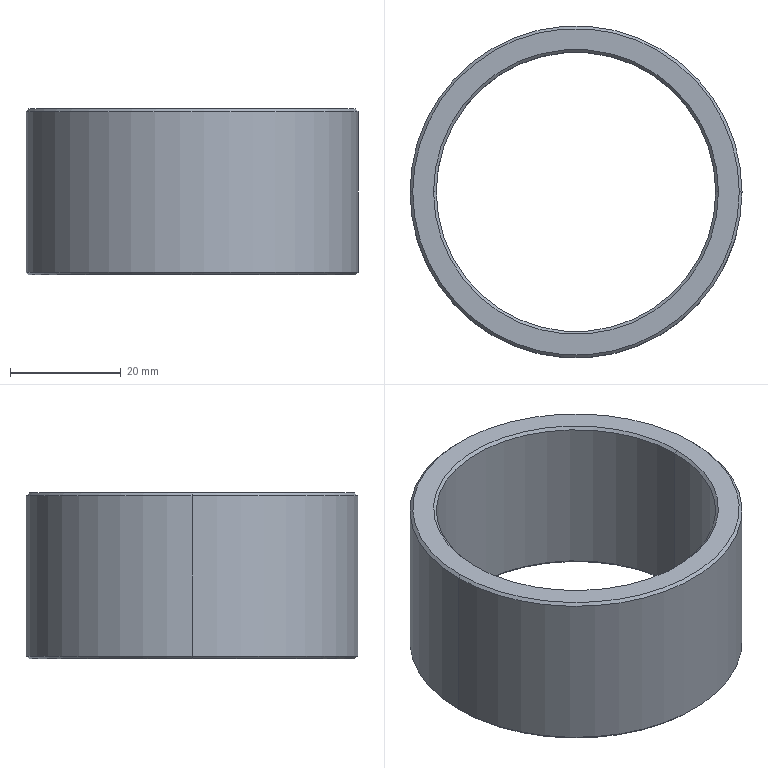Part | SolidWorks | features BaseBody 1 | 1 solid | 14 faces | box 60 x 60 x 30 mm | volume 24647 mm3 | cone 8 | cylinder 4 | plane 2 | commonest cylinder face diameters 50.5 x2 60 x2
STEP:
#1=CARTESIAN_POINT('',(-25.25,0.,14.5));
#2=VERTEX_POINT('',#1);
#3=CARTESIAN_POINT('',(25.25,0.,14.5));
#4=VERTEX_POINT('',#3);
#5=CARTESIAN_POINT('',(0.,0.,14.5));
#6=DIRECTION('',(0.,0.,1.));
#7=DIRECTION('',(1.,0.,0.));
#8=AXIS2_PLACEMENT_3D('',#5,#6,#7);
#9=CIRCLE('',#8,25.25);
#10=EDGE_CURVE('',#2,#4,#9,.T.);
#11=ORIENTED_EDGE('',*,*,#10,.F.);
#12=CARTESIAN_POINT('',(-25.75,0.,15.));
#13=VERTEX_POINT('',#12);
#14=CARTESIAN_POINT('',(-25.25,0.,14.5));
#15=DIRECTION('',(-0.7071,0.,0.7071));
#16=VECTOR('',#15,1000.);
#17=LINE('',#14,#16);
#18=EDGE_CURVE('',#2,#13,#17,.T.);
#19=ORIENTED_EDGE('',*,*,#18,.T.);
#20=CARTESIAN_POINT('',(25.75,0.,15.));
#21=VERTEX_POINT('',#20);
#22=CARTESIAN_POINT('',(0.,0.,15.));
#23=DIRECTION('',(0.,0.,-1.));
#24=DIRECTION('',(1.,0.,0.));
#25=AXIS2_PLACEMENT_3D('',#22,#23,#24);
#26=CIRCLE('',#25,25.75);
#27=EDGE_CURVE('',#21,#13,#26,.T.);
#28=ORIENTED_EDGE('',*,*,#27,.F.);
#29=CARTESIAN_POINT('',(25.25,0.,14.5));
#30=DIRECTION('',(0.7071,0.,0.7071));
#31=VECTOR('',#30,1000.);
#32=LINE('',#29,#31);
#33=EDGE_CURVE('',#4,#21,#32,.T.);
#34=ORIENTED_EDGE('',*,*,#33,.F.);
#35=EDGE_LOOP('',(#11,#19,#28,#34));
#36=FACE_OUTER_BOUND('',#35,.T.);
#37=CARTESIAN_POINT('',(0.,0.,14.5));
#38=DIRECTION('',(0.,0.,1.));
#39=DIRECTION('',(1.,0.,0.));
#40=AXIS2_PLACEMENT_3D('',#37,#38,#39);
#41=CONICAL_SURFACE('',#40,25.25,0.7854);
#42=ADVANCED_FACE('',(#36),#41,.F.);
#43=CARTESIAN_POINT('',(29.5,0.,15.));
#44=VERTEX_POINT('',#43);
#45=CARTESIAN_POINT('',(-29.5,0.,15.));
#46=VERTEX_POINT('',#45);
#47=CARTESIAN_POINT('',(0.,0.,15.));
#48=DIRECTION('',(0.,0.,1.));
#49=DIRECTION('',(1.,0.,0.));
#50=AXIS2_PLACEMENT_3D('',#47,#48,#49);
#51=CIRCLE('',#50,29.5);
#52=EDGE_CURVE('',#44,#46,#51,.T.);
#53=ORIENTED_EDGE('',*,*,#52,.F.);
#54=CARTESIAN_POINT('',(30.,0.,14.5));
#55=VERTEX_POINT('',#54);
#56=CARTESIAN_POINT('',(29.5,0.,15.));
#57=DIRECTION('',(0.7071,0.,-0.7071));
#58=VECTOR('',#57,1000.);
#59=LINE('',#56,#58);
#60=EDGE_CURVE('',#44,#55,#59,.T.);
#61=ORIENTED_EDGE('',*,*,#60,.T.);
#62=CARTESIAN_POINT('',(-30.,0.,14.5));
#63=VERTEX_POINT('',#62);
#64=CARTESIAN_POINT('',(0.,0.,14.5));
#65=DIRECTION('',(0.,0.,-1.));
#66=DIRECTION('',(1.,0.,0.));
#67=AXIS2_PLACEMENT_3D('',#64,#65,#66);
#68=CIRCLE('',#67,30.);
#69=EDGE_CURVE('',#63,#55,#68,.T.);
#70=ORIENTED_EDGE('',*,*,#69,.F.);
#71=CARTESIAN_POINT('',(-29.5,0.,15.));
#72=DIRECTION('',(-0.7071,0.,-0.7071));
#73=VECTOR('',#72,1000.);
#74=LINE('',#71,#73);
#75=EDGE_CURVE('',#46,#63,#74,.T.);
#76=ORIENTED_EDGE('',*,*,#75,.F.);
#77=EDGE_LOOP('',(#53,#61,#70,#76));
#78=FACE_OUTER_BOUND('',#77,.T.);
#79=CARTESIAN_POINT('',(0.,0.,15.));
#80=DIRECTION('',(0.,0.,-1.));
#81=DIRECTION('',(-1.,0.,0.));
#82=AXIS2_PLACEMENT_3D('',#79,#80,#81);
#83=CONICAL_SURFACE('',#82,29.5,0.7854);
#84=ADVANCED_FACE('',(#78),#83,.T.);
#85=CARTESIAN_POINT('',(25.25,0.,-14.5));
#86=VERTEX_POINT('',#85);
#87=CARTESIAN_POINT('',(-25.25,0.,-14.5));
#88=VERTEX_POINT('',#87);
#89=CARTESIAN_POINT('',(0.,0.,-14.5));
#90=DIRECTION('',(0.,0.,-1.));
#91=DIRECTION('',(1.,0.,0.));
#92=AXIS2_PLACEMENT_3D('',#89,#90,#91);
#93=CIRCLE('',#92,25.25);
#94=EDGE_CURVE('',#86,#88,#93,.T.);
#95=ORIENTED_EDGE('',*,*,#94,.F.);
#96=CARTESIAN_POINT('',(25.75,0.,-15.));
#97=VERTEX_POINT('',#96);
#98=CARTESIAN_POINT('',(25.75,0.,-15.));
#99=DIRECTION('',(0.7071,0.,-0.7071));
#100=VECTOR('',#99,1000.);
#101=LINE('',#98,#100);
#102=EDGE_CURVE('',#86,#97,#101,.T.);
#103=ORIENTED_EDGE('',*,*,#102,.T.);
#104=CARTESIAN_POINT('',(-25.75,0.,-15.));
#105=VERTEX_POINT('',#104);
#106=CARTESIAN_POINT('',(0.,0.,-15.));
#107=DIRECTION('',(0.,0.,1.));
#108=DIRECTION('',(1.,0.,0.));
#109=AXIS2_PLACEMENT_3D('',#106,#107,#108);
#110=CIRCLE('',#109,25.75);
#111=EDGE_CURVE('',#105,#97,#110,.T.);
#112=ORIENTED_EDGE('',*,*,#111,.F.);
#113=CARTESIAN_POINT('',(-25.75,0.,-15.));
#114=DIRECTION('',(-0.7071,0.,-0.7071));
#115=VECTOR('',#114,1000.);
#116=LINE('',#113,#115);
#117=EDGE_CURVE('',#88,#105,#116,.T.);
#118=ORIENTED_EDGE('',*,*,#117,.F.);
#119=EDGE_LOOP('',(#95,#103,#112,#118));
#120=FACE_OUTER_BOUND('',#119,.T.);
#121=CARTESIAN_POINT('',(0.,0.,-15.));
#122=DIRECTION('',(0.,0.,-1.));
#123=DIRECTION('',(-1.,0.,0.));
#124=AXIS2_PLACEMENT_3D('',#121,#122,#123);
#125=CONICAL_SURFACE('',#124,25.75,0.7854);
#126=ADVANCED_FACE('',(#120),#125,.F.);
#127=CARTESIAN_POINT('',(-29.5,0.,-15.));
#128=VERTEX_POINT('',#127);
#129=CARTESIAN_POINT('',(29.5,0.,-15.));
#130=VERTEX_POINT('',#129);
#131=CARTESIAN_POINT('',(0.,0.,-15.));
#132=DIRECTION('',(0.,0.,-1.));
#133=DIRECTION('',(1.,0.,0.));
#134=AXIS2_PLACEMENT_3D('',#131,#132,#133);
#135=CIRCLE('',#134,29.5);
#136=EDGE_CURVE('',#128,#130,#135,.T.);
#137=ORIENTED_EDGE('',*,*,#136,.F.);
#138=CARTESIAN_POINT('',(-30.,0.,-14.5));
#139=VERTEX_POINT('',#138);
#140=CARTESIAN_POINT('',(-30.,0.,-14.5));
#141=DIRECTION('',(-0.7071,0.,0.7071));
#142=VECTOR('',#141,1000.);
#143=LINE('',#140,#142);
#144=EDGE_CURVE('',#128,#139,#143,.T.);
#145=ORIENTED_EDGE('',*,*,#144,.T.);
#146=CARTESIAN_POINT('',(30.,0.,-14.5));
#147=VERTEX_POINT('',#146);
#148=CARTESIAN_POINT('',(0.,0.,-14.5));
#149=DIRECTION('',(0.,0.,1.));
#150=DIRECTION('',(1.,0.,0.));
#151=AXIS2_PLACEMENT_3D('',#148,#149,#150);
#152=CIRCLE('',#151,30.);
#153=EDGE_CURVE('',#147,#139,#152,.T.);
#154=ORIENTED_EDGE('',*,*,#153,.F.);
#155=CARTESIAN_POINT('',(30.,0.,-14.5));
#156=DIRECTION('',(0.7071,0.,0.7071));
#157=VECTOR('',#156,1000.);
#158=LINE('',#155,#157);
#159=EDGE_CURVE('',#130,#147,#158,.T.);
#160=ORIENTED_EDGE('',*,*,#159,.F.);
#161=EDGE_LOOP('',(#137,#145,#154,#160));
#162=FACE_OUTER_BOUND('',#161,.T.);
#163=CARTESIAN_POINT('',(0.,0.,-14.5));
#164=DIRECTION('',(0.,0.,1.));
#165=DIRECTION('',(1.,0.,0.));
#166=AXIS2_PLACEMENT_3D('',#163,#164,#165);
#167=CONICAL_SURFACE('',#166,30.,0.7854);
#168=ADVANCED_FACE('',(#162),#167,.T.);
#169=ORIENTED_EDGE('',*,*,#10,.T.);
#170=CARTESIAN_POINT('',(25.25,0.,15.));
#171=DIRECTION('',(0.,0.,-1.));
#172=VECTOR('',#171,1000.);
#173=LINE('',#170,#172);
#174=EDGE_CURVE('',#4,#86,#173,.T.);
#175=ORIENTED_EDGE('',*,*,#174,.T.);
#176=ORIENTED_EDGE('',*,*,#94,.T.);
#177=CARTESIAN_POINT('',(-25.25,0.,15.));
#178=DIRECTION('',(0.,0.,-1.));
#179=VECTOR('',#178,1000.);
#180=LINE('',#177,#179);
#181=EDGE_CURVE('',#2,#88,#180,.T.);
#182=ORIENTED_EDGE('',*,*,#181,.F.);
#183=EDGE_LOOP('',(#169,#175,#176,#182));
#184=FACE_OUTER_BOUND('',#183,.T.);
#185=CARTESIAN_POINT('',(0.,0.,15.));
#186=DIRECTION('',(0.,0.,-1.));
#187=DIRECTION('',(-1.,0.,0.));
#188=AXIS2_PLACEMENT_3D('',#185,#186,#187);
#189=CYLINDRICAL_SURFACE('',#188,25.25);
#190=ADVANCED_FACE('',(#184),#189,.F.);
#191=ORIENTED_EDGE('',*,*,#69,.T.);
#192=CARTESIAN_POINT('',(30.,0.,15.));
#193=DIRECTION('',(0.,0.,-1.));
#194=VECTOR('',#193,1000.);
#195=LINE('',#192,#194);
#196=EDGE_CURVE('',#55,#147,#195,.T.);
#197=ORIENTED_EDGE('',*,*,#196,.T.);
#198=ORIENTED_EDGE('',*,*,#153,.T.);
#199=CARTESIAN_POINT('',(-30.,0.,15.));
#200=DIRECTION('',(0.,0.,-1.));
#201=VECTOR('',#200,1000.);
#202=LINE('',#199,#201);
#203=EDGE_CURVE('',#63,#139,#202,.T.);
#204=ORIENTED_EDGE('',*,*,#203,.F.);
#205=EDGE_LOOP('',(#191,#197,#198,#204));
#206=FACE_OUTER_BOUND('',#205,.T.);
#207=CARTESIAN_POINT('',(0.,0.,15.));
#208=DIRECTION('',(0.,0.,-1.));
#209=DIRECTION('',(-1.,0.,0.));
#210=AXIS2_PLACEMENT_3D('',#207,#208,#209);
#211=CYLINDRICAL_SURFACE('',#210,30.);
#212=ADVANCED_FACE('',(#206),#211,.T.);
#213=CARTESIAN_POINT('',(0.,0.,15.));
#214=DIRECTION('',(0.,0.,1.));
#215=DIRECTION('',(1.,0.,0.));
#216=AXIS2_PLACEMENT_3D('',#213,#214,#215);
#217=CIRCLE('',#216,29.5);
#218=EDGE_CURVE('',#46,#44,#217,.T.);
#219=ORIENTED_EDGE('',*,*,#218,.T.);
#220=ORIENTED_EDGE('',*,*,#52,.T.);
#221=EDGE_LOOP('',(#219,#220));
#222=FACE_OUTER_BOUND('',#221,.T.);
#223=ORIENTED_EDGE('',*,*,#27,.T.);
#224=CARTESIAN_POINT('',(0.,0.,15.));
#225=DIRECTION('',(0.,0.,-1.));
#226=DIRECTION('',(1.,0.,0.));
#227=AXIS2_PLACEMENT_3D('',#224,#225,#226);
#228=CIRCLE('',#227,25.75);
#229=EDGE_CURVE('',#13,#21,#228,.T.);
#230=ORIENTED_EDGE('',*,*,#229,.T.);
#231=EDGE_LOOP('',(#223,#230));
#232=FACE_BOUND('',#231,.T.);
#233=CARTESIAN_POINT('',(0.,0.,15.));
#234=DIRECTION('',(0.,0.,1.));
#235=DIRECTION('',(1.,0.,0.));
#236=AXIS2_PLACEMENT_3D('',#233,#234,#235);
#237=PLANE('',#236);
#238=ADVANCED_FACE('',(#222,#232),#237,.T.);
#239=CARTESIAN_POINT('',(0.,0.,-15.));
#240=DIRECTION('',(0.,0.,-1.));
#241=DIRECTION('',(1.,0.,0.));
#242=AXIS2_PLACEMENT_3D('',#239,#240,#241);
#243=CIRCLE('',#242,29.5);
#244=EDGE_CURVE('',#130,#128,#243,.T.);
#245=ORIENTED_EDGE('',*,*,#244,.T.);
#246=ORIENTED_EDGE('',*,*,#136,.T.);
#247=EDGE_LOOP('',(#245,#246));
#248=FACE_OUTER_BOUND('',#247,.T.);
#249=ORIENTED_EDGE('',*,*,#111,.T.);
#250=CARTESIAN_POINT('',(0.,0.,-15.));
#251=DIRECTION('',(0.,0.,1.));
#252=DIRECTION('',(1.,0.,0.));
#253=AXIS2_PLACEMENT_3D('',#250,#251,#252);
#254=CIRCLE('',#253,25.75);
#255=EDGE_CURVE('',#97,#105,#254,.T.);
#256=ORIENTED_EDGE('',*,*,#255,.T.);
#257=EDGE_LOOP('',(#249,#256));
#258=FACE_BOUND('',#257,.T.);
#259=CARTESIAN_POINT('',(0.,0.,-15.));
#260=DIRECTION('',(0.,0.,1.));
#261=DIRECTION('',(1.,0.,0.));
#262=AXIS2_PLACEMENT_3D('',#259,#260,#261);
#263=PLANE('',#262);
#264=ADVANCED_FACE('',(#248,#258),#263,.F.);
#265=ORIENTED_EDGE('',*,*,#196,.F.);
#266=CARTESIAN_POINT('',(0.,0.,14.5));
#267=DIRECTION('',(0.,0.,-1.));
#268=DIRECTION('',(1.,0.,0.));
#269=AXIS2_PLACEMENT_3D('',#266,#267,#268);
#270=CIRCLE('',#269,30.);
#271=EDGE_CURVE('',#55,#63,#270,.T.);
#272=ORIENTED_EDGE('',*,*,#271,.T.);
#273=ORIENTED_EDGE('',*,*,#203,.T.);
#274=CARTESIAN_POINT('',(0.,0.,-14.5));
#275=DIRECTION('',(0.,0.,1.));
#276=DIRECTION('',(1.,0.,0.));
#277=AXIS2_PLACEMENT_3D('',#274,#275,#276);
#278=CIRCLE('',#277,30.);
#279=EDGE_CURVE('',#139,#147,#278,.T.);
#280=ORIENTED_EDGE('',*,*,#279,.T.);
#281=EDGE_LOOP('',(#265,#272,#273,#280));
#282=FACE_OUTER_BOUND('',#281,.T.);
#283=CARTESIAN_POINT('',(0.,0.,15.));
#284=DIRECTION('',(0.,0.,-1.));
#285=DIRECTION('',(-1.,0.,0.));
#286=AXIS2_PLACEMENT_3D('',#283,#284,#285);
#287=CYLINDRICAL_SURFACE('',#286,30.);
#288=ADVANCED_FACE('',(#282),#287,.T.);
#289=ORIENTED_EDGE('',*,*,#174,.F.);
#290=CARTESIAN_POINT('',(0.,0.,14.5));
#291=DIRECTION('',(0.,0.,1.));
#292=DIRECTION('',(1.,0.,0.));
#293=AXIS2_PLACEMENT_3D('',#290,#291,#292);
#294=CIRCLE('',#293,25.25);
#295=EDGE_CURVE('',#4,#2,#294,.T.);
#296=ORIENTED_EDGE('',*,*,#295,.T.);
#297=ORIENTED_EDGE('',*,*,#181,.T.);
#298=CARTESIAN_POINT('',(0.,0.,-14.5));
#299=DIRECTION('',(0.,0.,-1.));
#300=DIRECTION('',(1.,0.,0.));
#301=AXIS2_PLACEMENT_3D('',#298,#299,#300);
#302=CIRCLE('',#301,25.25);
#303=EDGE_CURVE('',#88,#86,#302,.T.);
#304=ORIENTED_EDGE('',*,*,#303,.T.);
#305=EDGE_LOOP('',(#289,#296,#297,#304));
#306=FACE_OUTER_BOUND('',#305,.T.);
#307=CARTESIAN_POINT('',(0.,0.,15.));
#308=DIRECTION('',(0.,0.,-1.));
#309=DIRECTION('',(-1.,0.,0.));
#310=AXIS2_PLACEMENT_3D('',#307,#308,#309);
#311=CYLINDRICAL_SURFACE('',#310,25.25);
#312=ADVANCED_FACE('',(#306),#311,.F.);
#313=ORIENTED_EDGE('',*,*,#144,.F.);
#314=ORIENTED_EDGE('',*,*,#244,.F.);
#315=ORIENTED_EDGE('',*,*,#159,.T.);
#316=ORIENTED_EDGE('',*,*,#279,.F.);
#317=EDGE_LOOP('',(#313,#314,#315,#316));
#318=FACE_OUTER_BOUND('',#317,.T.);
#319=CARTESIAN_POINT('',(0.,0.,-14.5));
#320=DIRECTION('',(0.,0.,1.));
#321=DIRECTION('',(1.,0.,0.));
#322=AXIS2_PLACEMENT_3D('',#319,#320,#321);
#323=CONICAL_SURFACE('',#322,30.,0.7854);
#324=ADVANCED_FACE('',(#318),#323,.T.);
#325=ORIENTED_EDGE('',*,*,#102,.F.);
#326=ORIENTED_EDGE('',*,*,#303,.F.);
#327=ORIENTED_EDGE('',*,*,#117,.T.);
#328=ORIENTED_EDGE('',*,*,#255,.F.);
#329=EDGE_LOOP('',(#325,#326,#327,#328));
#330=FACE_OUTER_BOUND('',#329,.T.);
#331=CARTESIAN_POINT('',(0.,0.,-15.));
#332=DIRECTION('',(0.,0.,-1.));
#333=DIRECTION('',(-1.,0.,0.));
#334=AXIS2_PLACEMENT_3D('',#331,#332,#333);
#335=CONICAL_SURFACE('',#334,25.75,0.7854);
#336=ADVANCED_FACE('',(#330),#335,.F.);
#337=ORIENTED_EDGE('',*,*,#60,.F.);
#338=ORIENTED_EDGE('',*,*,#218,.F.);
#339=ORIENTED_EDGE('',*,*,#75,.T.);
#340=ORIENTED_EDGE('',*,*,#271,.F.);
#341=EDGE_LOOP('',(#337,#338,#339,#340));
#342=FACE_OUTER_BOUND('',#341,.T.);
#343=CARTESIAN_POINT('',(0.,0.,15.));
#344=DIRECTION('',(0.,0.,-1.));
#345=DIRECTION('',(-1.,0.,0.));
#346=AXIS2_PLACEMENT_3D('',#343,#344,#345);
#347=CONICAL_SURFACE('',#346,29.5,0.7854);
#348=ADVANCED_FACE('',(#342),#347,.T.);
#349=ORIENTED_EDGE('',*,*,#18,.F.);
#350=ORIENTED_EDGE('',*,*,#295,.F.);
#351=ORIENTED_EDGE('',*,*,#33,.T.);
#352=ORIENTED_EDGE('',*,*,#229,.F.);
#353=EDGE_LOOP('',(#349,#350,#351,#352));
#354=FACE_OUTER_BOUND('',#353,.T.);
#355=CARTESIAN_POINT('',(0.,0.,14.5));
#356=DIRECTION('',(0.,0.,1.));
#357=DIRECTION('',(1.,0.,0.));
#358=AXIS2_PLACEMENT_3D('',#355,#356,#357);
#359=CONICAL_SURFACE('',#358,25.25,0.7854);
#360=ADVANCED_FACE('',(#354),#359,.F.);
#361=CLOSED_SHELL('',(#42,#84,#126,#168,#190,#212,#238,#264,#288,#312,#324,#336,#348,#360));
#362=MANIFOLD_SOLID_BREP('',#361);
#363=CARTESIAN_POINT('',(0.,0.,0.));
#364=DIRECTION('',(0.,0.,1.));
#365=DIRECTION('',(1.,0.,0.));
#366=AXIS2_PLACEMENT_3D('',#363,#364,#365);
#367=(LENGTH_UNIT()NAMED_UNIT(*)SI_UNIT(.MILLI.,.METRE.));
#368=UNCERTAINTY_MEASURE_WITH_UNIT(LENGTH_MEASURE(0.00001),#367,'','');
#369=(NAMED_UNIT(*)PLANE_ANGLE_UNIT()SI_UNIT($,.RADIAN.));
#370=(NAMED_UNIT(*)SI_UNIT($,.STERADIAN.)SOLID_ANGLE_UNIT());
#371=(GEOMETRIC_REPRESENTATION_CONTEXT(3)GLOBAL_UNCERTAINTY_ASSIGNED_CONTEXT((#368))GLOBAL_UNIT_ASSIGNED_CONTEXT((#367,#369,#370))REPRESENTATION_CONTEXT('',''));
#372=ADVANCED_BREP_SHAPE_REPRESENTATION('',(#362,#366),#371);